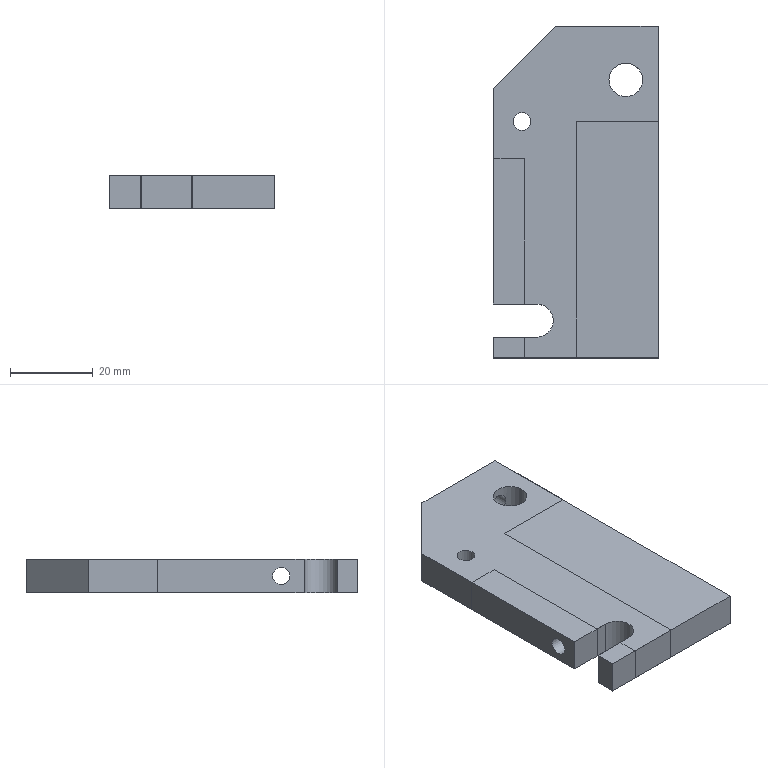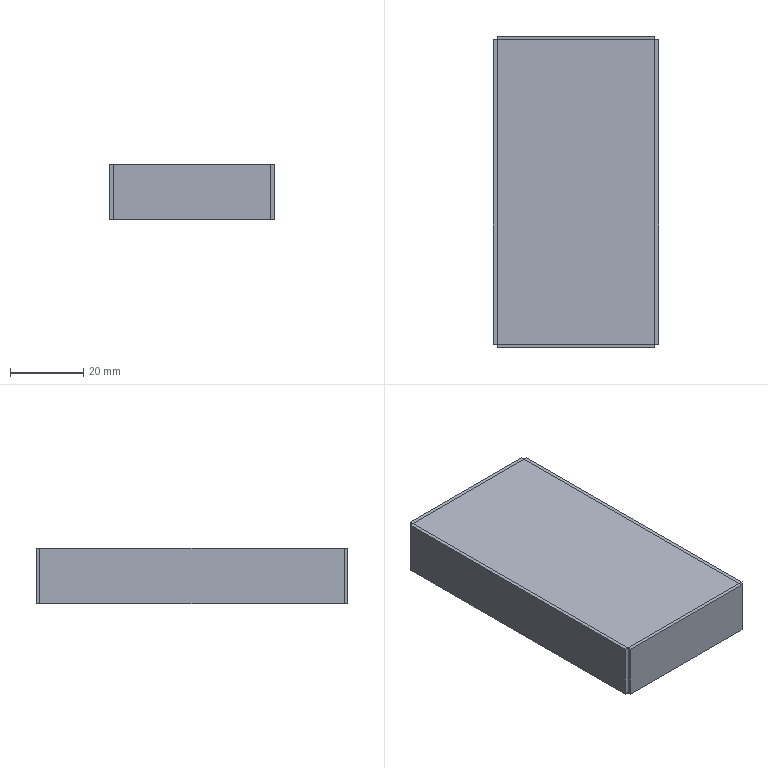CAM job | NX | 3+2 milling, drilling | part box 40 x 80 x 8 mm | stock box 45 x 85 x 15 mm
Tools:
number,name,description,diameter,corner_radius,flute_length,length,flutes
11,D4-12-D4-50-3T-FINISH,D4-12-D4-50-3T,4.0,0.0,12.0,50.0,3
4,D5-15-D6-50-3T-ROUGH,D5-15-D6-50-3T,5.0,0.0,15.0,16.0,3
6,D6-18-D6-50-3T-FINISH,D6-18-D6-50-3T,6.0,0.0,18.0,50.0,3
1,D10-30-D10-75-3T-ROUGH,D10-30-D10-75-3T-粗,10.0,0.0,30.0,75.0,2
10,D63面刀,D63面刀,63.0,0.0,30.0,30.0,4
13,钻头D4.3-54-83,钻刀D4.3-54-83,4.3,0.0,54.0,83.0,2
12,上排M5-22-D5.5-60,上排M5-22-D5.5-60,5.0,0.0,22.0,25.0,2
5,倒角D4-90度,倒角D4-90度,4.0,0.0,5.0,50.0,2
2,倒角D10-90度,倒角D10-90度,10.0,0.0,10.0,75.0,2
Operations:
program,operation,operation_type,tool,method,geometry_group,spindle_rpm,surface_speed,feed_per_tooth,feed_cut,feed_plunge,cut_length_mm,path_length_mm,cut_time_min,machine_time_min
A1,FLOOR_FACING_1,VolumeBased25DMillingOperation,D63面刀,METHOD,A-G54,1600.0,316.0,0.0938,600.0,100.0,155.0,189.0,0.2583,0.2617
A1,动态粗,CavityMilling,D10-30-D10-75-3T-ROUGH,METHOD,WORKPIECE_54,3500.0,109.0,0.2143,1500.0,100.0,2914.997,2973.997,1.782,1.788
A1,DRILLING,Operation,倒角D10-90度,METHOD,WORKPIECE_54,1200.0,37.0,0.025,60.0,0.0,11.0,92.092,0.1833,0.1914
A1,DRILLING_COPY,Operation,钻头D4.3-54-83,METHOD,WORKPIECE_54,1600.0,21.0,0.0187,60.0,0.0,30.0,130.092,0.5,0.51
A1,动态粗_COPY,CavityMilling,D5-15-D6-50-3T-ROUGH,METHOD,WORKPIECE_54,3000.0,47.0,0.1111,1000.0,100.0,2268.985,2387.258,2.182,2.194
A1,PLANAR_MILL,PlanarMilling,D5-15-D6-50-3T-ROUGH,METHOD,WORKPIECE_54,3500.0,100.0,0.1178,800.0,100.0,220.605,268.605,0.2758,0.2806
A1,PLANAR_MILL_COPY,PlanarMilling,D4-12-D4-50-3T-FINISH,METHOD,WORKPIECE_54,3000.0,37.0,0.0333,300.0,100.0,39.504,95.504,0.1317,0.1373
A1,DRILLING_1,Operation,上排M5-22-D5.5-60,METHOD,WORKPIECE_54,300.0,4.0,0.0013,0.8,0.0,8.0,56.0,10.0,10.005
A1,PLANAR_MILL_1,PlanarMilling,倒角D4-90度,METHOD,WORKPIECE_54,3000.0,37.0,0.1333,800.0,100.0,272.149,310.149,0.3402,0.344
A1,PLANAR_MILL_2,PlanarMilling,倒角D4-90度,METHOD,WORKPIECE_54,3000.0,37.0,0.1333,800.0,100.0,27.826,65.826,0.0348,0.0386
A1,PLANAR_MILL_3,PlanarMilling,D6-18-D6-50-3T-FINISH,METHOD,WORKPIECE_54,3000.0,56.0,0.0667,600.0,100.0,569.258,623.258,0.9488,0.9542
A1,FLOOR_FACING_1_COPY,VolumeBased25DMillingOperation,D63面刀,METHOD,A-G54,1600.0,316.0,0.0938,600.0,100.0,155.0,189.0,0.2583,0.2617
B1,ADAPTIVE_MILLING,CavityMilling,D10-30-D10-75-3T-ROUGH,METHOD,WORKPIECE_55,3000.0,94.0,0.25,1500.0,100.0,9390.925,9424.726,6.261,6.264
B1,PLANAR_MILL_4,PlanarMilling,D63面刀,METHOD,WORKPIECE_55,1600.0,316.0,0.0938,600.0,100.0,155.0,189.0,0.2583,0.2617
B1,PLANAR_MILL_5,PlanarMilling,倒角D4-90度,METHOD,WORKPIECE_55,3000.0,37.0,0.1333,800.0,100.0,274.346,312.346,0.3429,0.3467
B1,PLANAR_MILL_5_COPY,PlanarMilling,倒角D4-90度,METHOD,WORKPIECE_55,3000.0,37.0,0.1333,800.0,100.0,27.826,65.826,0.0348,0.0386
B1,PLANAR_MILL_5_COPY_COPY,PlanarMilling,倒角D4-90度,METHOD,WORKPIECE_55,3000.0,37.0,0.1333,800.0,100.0,14.266,52.266,0.0178,0.0216
C1,DRILLING_2,Operation,倒角D10-90度,METHOD,C-G56,1200.0,37.0,0.025,60.0,0.0,4.0,11.0,0.0667,0.0674
C1,DRILLING_2_COPY,Operation,钻头D4.3-54-83,METHOD,C-G56,1300.0,17.0,0.0231,60.0,0.0,18.0,39.0,0.3,0.3021
C1,DRILLING_2_COPY_1,Operation,倒角D10-90度,METHOD,C-G56,2000.0,62.0,0.03,120.0,0.0,5.5,14.0,0.0458,0.0467
C1,DRILLING_2_COPY_COPY,Operation,上排M5-22-D5.5-60,METHOD,C-G56,300.0,4.0,0.0013,0.8,0.0,8.0,19.0,10.0,10.001
D1,FLOOR_FACING,VolumeBased25DMillingOperation,D10-30-D10-75-3T-ROUGH,METHOD,D-G57,3000.0,94.0,0.25,1500.0,100.0,4492.5,6665.686,2.995,3.212
D1,FLOOR_FACING_COPY,VolumeBased25DMillingOperation,D6-18-D6-50-3T-FINISH,METHOD,D-G57,3000.0,100.0,0.1178,600.0,100.0,209.3,258.5,0.3488,0.3538
D1,FLOOR_FACING_COPY_COPY,VolumeBased25DMillingOperation,D6-18-D6-50-3T-FINISH,METHOD,D-G57,3000.0,100.0,0.1178,600.0,100.0,26.0,75.2,0.0433,0.0483
D1,PLANAR_MILL_6_COPY,PlanarMilling,倒角D4-90度,METHOD,D-G57,3000.0,37.0,0.1333,800.0,100.0,60.0,235.6,0.075,0.0926
D1,PLANAR_MILL_6,PlanarMilling,倒角D4-90度,METHOD,D-G57,3000.0,37.0,0.1333,800.0,100.0,20.0,59.0,0.025,0.0289
E1,FLOOR_FACING_COPY_1,VolumeBased25DMillingOperation,D10-30-D10-75-3T-ROUGH,METHOD,E-G58,3000.0,94.0,0.25,1500.0,100.0,13862.299,20747.299,9.242,9.93
E1,PLANAR_MILL_7,PlanarMilling,倒角D4-90度,METHOD,E-G58,3000.0,37.0,0.1333,800.0,100.0,22.0,59.0,0.0275,0.0312
E1,PLANAR_MILL_7_COPY,PlanarMilling,倒角D4-90度,METHOD,E-G58,3000.0,37.0,0.1333,800.0,100.0,22.0,99.0,0.0275,0.0352
E1,DRILLING_3,Operation,倒角D10-90度,METHOD,E-G58,1200.0,37.0,0.025,60.0,0.0,5.5,91.0,0.0917,0.1002
E1,DRILLING_4,Operation,钻头D4.3-54-83,METHOD,E-G58,1600.0,21.0,0.0187,60.0,0.0,19.0,118.0,0.3167,0.3266
E1,DRILLING_4_COPY,Operation,上排M5-22-D5.5-60,METHOD,E-G58,300.0,4.0,0.0013,0.8,0.0,8.0,96.0,10.0,10.009
E1,FLOOR_FACING_COPY_1_COPY_COPY,VolumeBased25DMillingOperation,D6-18-D6-50-3T-FINISH,METHOD,E-G58,3000.0,56.0,0.0667,600.0,100.0,52.0,200.0,0.0867,0.1015
E1,FLOOR_FACING_COPY_1_COPY,VolumeBased25DMillingOperation,D6-18-D6-50-3T-FINISH,METHOD,E-G58,3000.0,56.0,0.0667,600.0,100.0,246.3,320.3,0.4105,0.4179